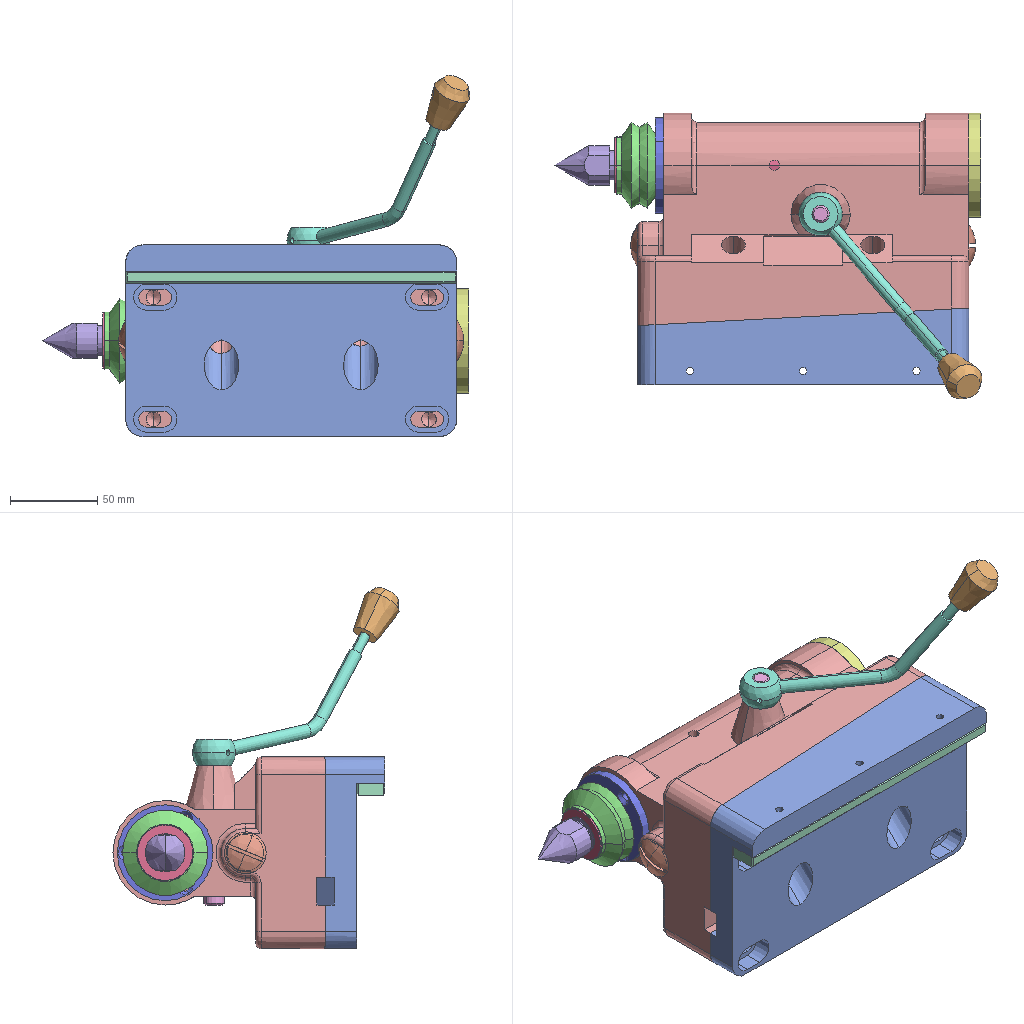Assembly | SolidWorks | 16 different items | 17 placed | box 245 x 164 x 207 mm
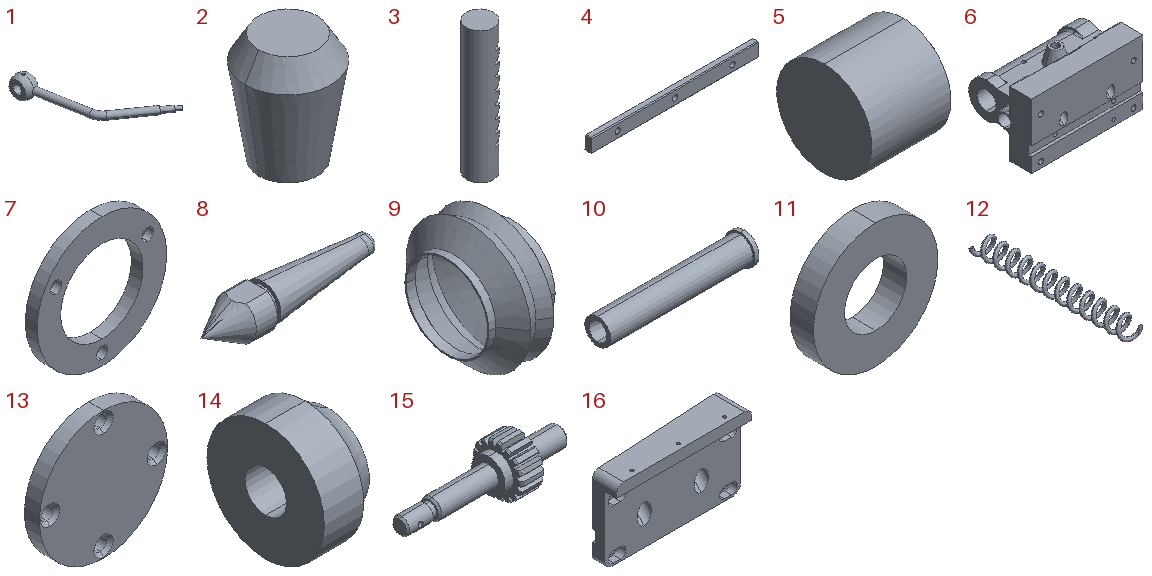Parts list (item | quantity | size | volume | features):
1 | x1 | 81.686 x 132.115 x 24.819 mm | 11563 mm3 | features ICE 4, Revolution 1, StudWizard 1, Sweep 1, SweepCut 1
2 | x1 | 22 x 22 x 28 mm | 7214 mm3 | features HoleWzd 1, Revolution 1
3 | x1 | 18 x 18 x 88 mm | 19025 mm3 | features ICE 2, Extrusion 1, LPattern 1
4 | x1 | 190 x 7 x 16 mm | 20157 mm3 | features Chamfer 1, Extrusion 1, HoleWzd 1
5 | x2 | 23.975 x 24 x 24 mm | 9856 mm3 | features ICE 1, Revolution 1
6 | x1 | 190 x 122 x 110 mm | 1237732 mm3 | features ICE 19, HoleWzd 6, Fillet 3, Extrusion 1, Revolution 1
7 | x1 | 55 x 5 x 55 mm | 6655 mm3 | features Extrusion 1, HoleWzd 1
8 | x1 | 94.92 x 23 x 21 mm | 19307 mm3 | features Fillet 1, ICE 1, Revolution 1
9 | x1 | 26 x 49 x 49 mm | 4109 mm3 | features ICE 1, RevCut 1, Revolution 1
10 | x1 | 180 x 37 x 37 mm | 98767 mm3 | features ICE 4, Extrusion 1, RevCut 1
11 | x1 | 16 x 3 x 16 mm | 452.389 mm3 | features Extrusion 1
12 | x1 | 17 x 130 x 17 mm | 3869 mm3 | features ICE 1, Sweep 1
13 | x1 | 60 x 20 x 60 mm | 17734 mm3 | features ICE 2, Extrusion 1, Fillet 1, HoleWzd 1
14 | x1 | 18 x 34 x 34 mm | 12469 mm3 | features ICE 1, Revolution 1
15 | x1 | 95 x 29.923 x 29.999 mm | 17712 mm3 | features ICE 7, Chamfer 1, CirPattern 1, Extrusion 1, SweepCut 1
16 | x1 | 190 x 44 x 110 mm | 466301 mm3 | features ICE 4, Extrusion 1, Fillet 1, HoleWzd 1, MirrorPattern 1, SweepCut 1
Mates (type | each side: item.copy, entity, surface, feature):
Coincident | 6.1 plane | assembly plane | 3 times
Coincident | 6.1 face plane | 16.1 face plane Boss-Extrude1 | 2 times
Coincident | 6.1 face plane Cut-Extrude1 | 16.1 face plane Boss-Extrude1
Concentric | 1.1 face cylinder Boss-Extrude2 | 2.1 face cylinder M6 Tapped Hole1
Coincident | 1.1 face plane Boss-Extrude1 | 2.1 face plane Revolve1
Concentric | 15.1 face cylinder Boss-Extrude1 | 1.1 face cylinder Cut-Extrude2
Concentric | 15.1 face cylinder Cut-Sweep1 | 1.1 face cylinder Cut-Sweep1
Concentric | 14.1 face cylinder Cut-Extrude1 | 15.1 face cylinder Boss-Extrude7
Coincident | 14.1 face plane Revolve1 | 15.1 face plane Boss-Extrude5
Concentric | 6.1 face cylinder | 15.1 face cylinder Boss-Extrude3
Coincident | 6.1 face plane | 1.1 face plane Cut-Extrude1
Concentric | 8.1 face cylinder Revolve1 | 10.1 face cylinder Cut-Extrude1
Concentric | 8.1 face cylinder Revolve1 | 9.1 face cylinder Revolve1
Coincident | 8.1 face plane Revolve1 | 10.1 face plane Boss-Extrude1
Concentric | 10.1 face cylinder Cut-Extrude1 | 11.1 face cylinder Boss-Extrude1
Concentric | 8.1 face cylinder Revolve1 | assembly face
Coincident | assembly face | 10.1 face plane Boss-Extrude1
Coincident | assembly face | 9.1 face plane Revolve1
Coincident | 10.1 face plane Cut-Extrude1 | 11.1 face plane Boss-Extrude1
Concentric | 6.1 face cylinder | 10.1 face cylinder Boss-Extrude1
Coincident | 16.1 face plane Cut-Extrude2 | assembly face | 2 times
Concentric | 6.1 face cylinder | 13.1 face cylinder Boss-Extrude2
Concentric | 6.1 face cylinder | assembly face | 9 times
Coincident | 6.1 face plane | assembly face | 3 times
Concentric | 6.1 face cylinder | 3.1 face cylinder Boss-Extrude1
Concentric | 6.1 face cylinder | 5.1 face cylinder Revolve1
Coincident | 6.1 face plane | 5.1 face plane Cut-Extrude1
Concentric | 10.1 face cylinder Boss-Extrude1 | 7.1 face cylinder Boss-Extrude1
Concentric | 6.1 face cylinder | 7.1 face cylinder Hole1
Coincident | 6.1 face plane | 7.1 face plane Boss-Extrude1
Concentric | 6.1 face cylinder | 13.1 face cylinder Hole1
Coincident | 6.1 edge | 13.1 face plane Boss-Extrude1
Concentric | 16.1 edge | 4.1 face cylinder Hole1
Concentric | 16.1 face cylinder M5 Tapped Hole1 | 4.1 face cylinder Hole1
Coincident | 16.1 face plane Cut-Extrude1 | 4.1 face plane Boss-Extrude1
Concentric | 6.1 face cylinder | 12.1 select_type:24
Concentric | 6.1 face cylinder | assembly select_type:0
Coincident | 6.1 face plane | 10.1 face plane Boss-Extrude2
Coincident | 6.1 face plane | 12.1 face plane Cut-Extrude1
Coincident | 16.1 face plane Cut-Extrude3 | assembly face | 4 times
Concentric | assembly face | assembly face | 4 times
Coincident | assembly face | assembly face | 5 times
Concentric | 4.1 face cylinder Hole1 | assembly face | 3 times
Parallel | 4.1 face cone Hole1 | assembly face
Coincident | 4.1 face cone Hole1 | assembly face | 3 times
Concentric | 6.1 face cylinder | 5.2 face cylinder Revolve1
Coincident | 6.1 face plane | 5.2 edge